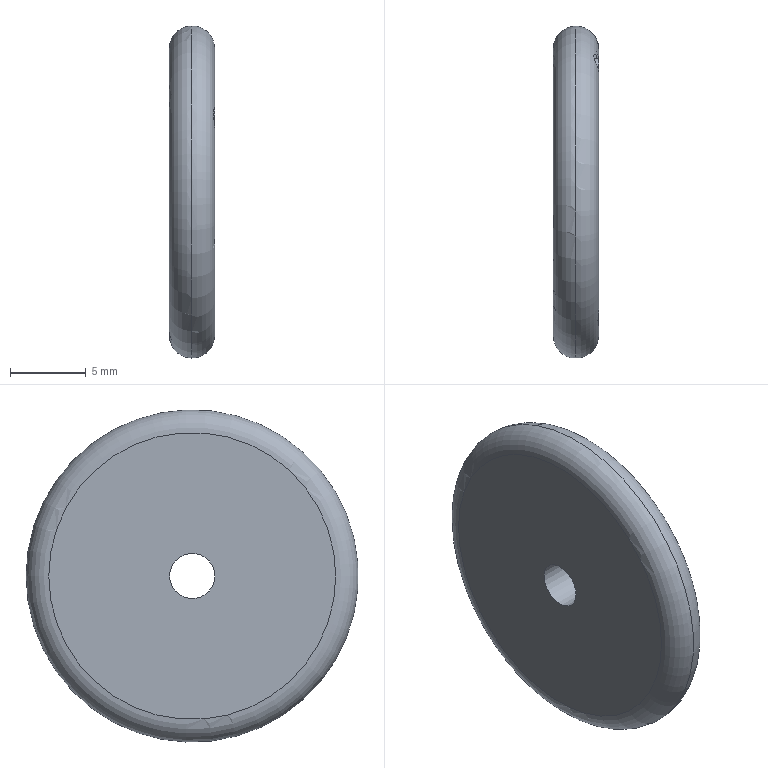Part | STEP file | 1-75.7 | 1 solid | 158 faces | box 3 x 22 x 22 mm | volume 1050 mm3 | spline 84 | plane 70 | cylinder 2 | torus 2 | commonest cylinder face diameters 0.301 x1 3 x1